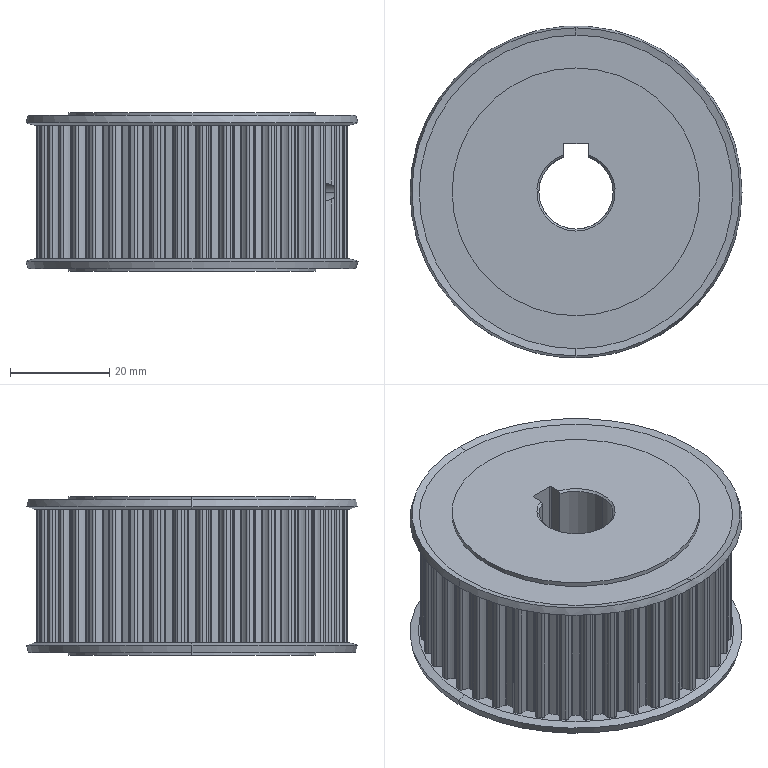Part | SolidWorks | features BaseBody 1 | 1 solid | 407 faces | box 67 x 67 x 32 mm | volume 86372 mm3 | cylinder 381 | cone 17 | plane 9 | commonest cylinder face diameters 1.1 x99 0.5 x96 6.55 x90 59.16 x43 62.7 x40 4.134 x4